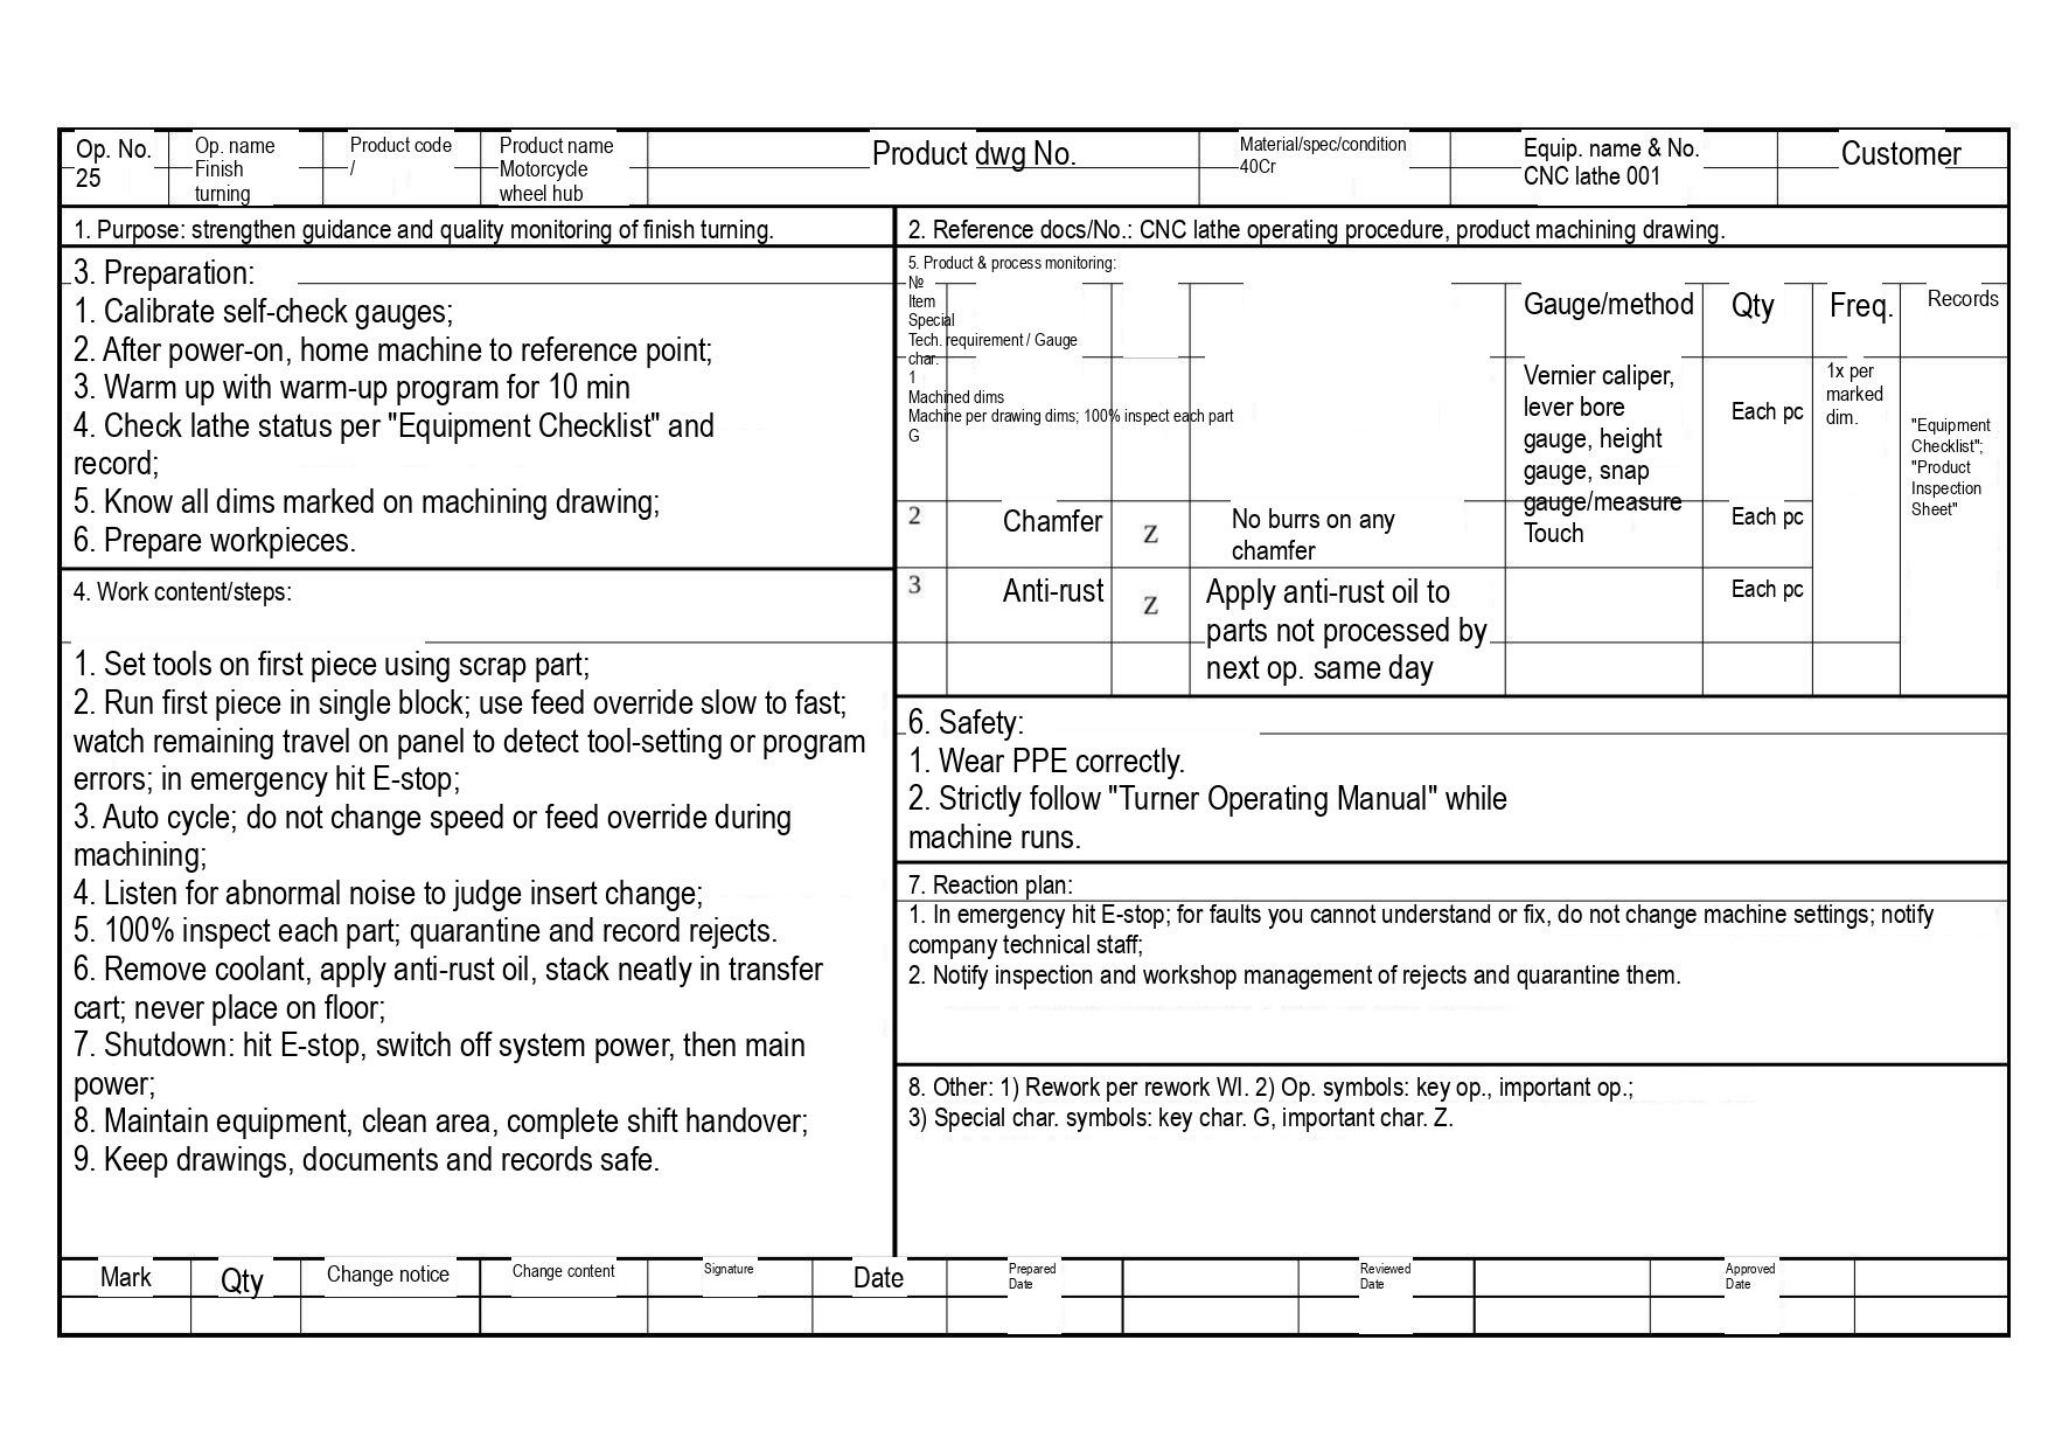| Op. No. 25 | Op. name Finish turning | Product code / | Product name Motorcycle wheel hub | Product dwg No. | Material/spec/condition 40Cr | Equip. name & No. CNC lathe 001 | Customer |
|---|---|---|---|---|---|---|---|

1. Purpose: strengthen guidance and quality monitoring of finish turning.

2. Reference docs/No.: CNC lathe operating procedure, product machining drawing.

3. Preparation:
1. Calibrate self-check gauges;
2. After power-on, home machine to reference point;
3. Warm up with warm-up program for 10 min
4. Check lathe status per "Equipment Checklist" and record;
5. Know all dims marked on machining drawing;
6. Prepare workpieces.

4. Work content/steps:

1. Set tools on first piece using scrap part;
2. Run first piece in single block; use feed override slow to fast; watch remaining travel on panel to detect tool-setting or program errors; in emergency hit E-stop;
3. Auto cycle; do not change speed or feed override during machining;
4. Listen for abnormal noise to judge insert change;
5. 100% inspect each part; quarantine and record rejects.
6. Remove coolant, apply anti-rust oil, stack neatly in transfer cart; never place on floor;
7. Shutdown: hit E-stop, switch off system power, then main power;
8. Maintain equipment, clean area, complete shift handover;
9. Keep drawings, documents and records safe.

5. Product & process monitoring:

| № | Item | Special char. | Tech. requirement / Gauge | Gauge/method | Qty | Freq. | Records |
|---|---|---|---|---|---|---|---|
| 1 | Machined dims | G | Machine per drawing dims; 100% inspect each part | Vernier caliper, lever bore gauge, height gauge, snap gauge/measure Touch | Each pc | 1x per marked dim. | "Equipment Checklist"; "Product Inspection Sheet" |
| 2 | Chamfer | Z | No burrs on any chamfer | | Each pc | | |
| 3 | Anti-rust | Z | Apply anti-rust oil to parts not processed by next op. same day | | Each pc | | |

6. Safety:
1. Wear PPE correctly.
2. Strictly follow "Turner Operating Manual" while machine runs.

7. Reaction plan:
1. In emergency hit E-stop; for faults you cannot understand or fix, do not change machine settings; notify company technical staff;
2. Notify inspection and workshop management of rejects and quarantine them.

8. Other: 1) Rework per rework WI. 2) Op. symbols: key op., important op.;
3) Special char. symbols: key char. G, important char. Z.

| Mark | Qty | Change notice | Change content | Signature | Date | Prepared Date | | Reviewed Date | | Approved Date | |
|---|---|---|---|---|---|---|---|---|---|---|---|
| | | | | | | | | | | | |